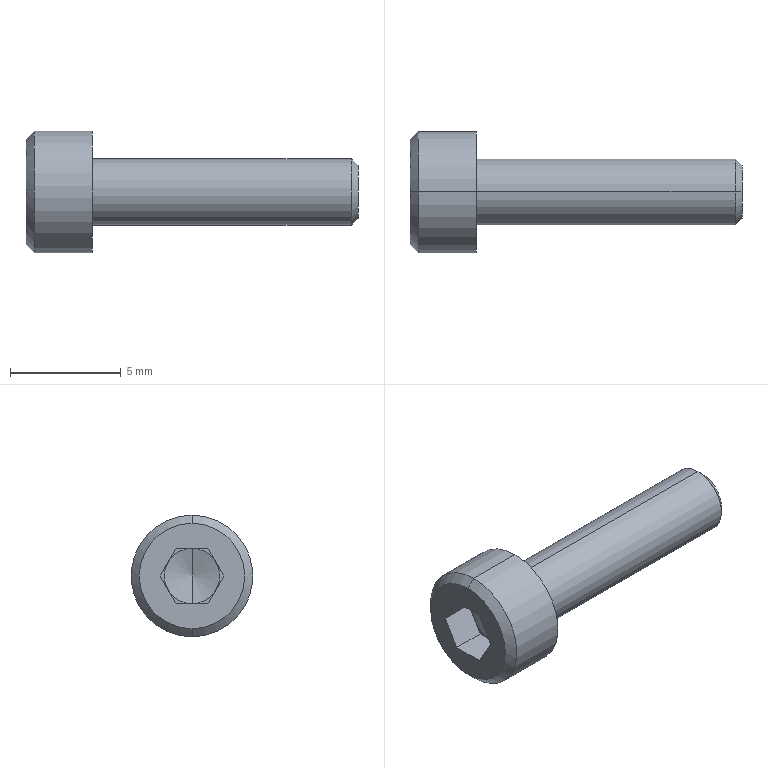Part | SolidWorks | features ICE 1, RevCut 1, Revolution 1 | 1 solid | 25 faces | box 15 x 5.5 x 5.5 mm | volume 145.907 mm3 | plane 15 | cone 6 | cylinder 4 | commonest cylinder face diameters 3 x2 5.5 x2